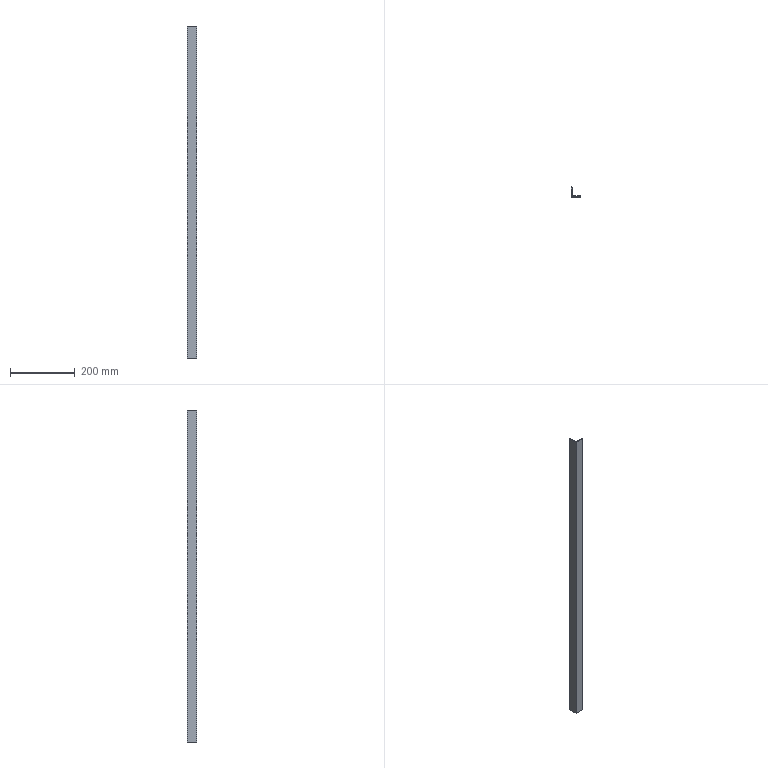Part | SolidWorks | features Extrusion 1 | 1 solid | 11 faces | box 30 x 30 x 1024 mm | volume 174225 mm3 | plane 8 | cylinder 3 | commonest cylinder face diameters 4 x3
STEP:
#1=CARTESIAN_POINT('',(0.,30.,0.));
#2=VERTEX_POINT('',#1);
#3=CARTESIAN_POINT('',(0.,0.,0.));
#4=VERTEX_POINT('',#3);
#5=CARTESIAN_POINT('',(0.,0.,0.));
#6=DIRECTION('',(0.,-1.,0.));
#7=VECTOR('',#6,1000.);
#8=LINE('',#5,#7);
#9=EDGE_CURVE('',#2,#4,#8,.T.);
#10=ORIENTED_EDGE('',*,*,#9,.T.);
#11=CARTESIAN_POINT('',(0.,0.,1024.));
#12=VERTEX_POINT('',#11);
#13=CARTESIAN_POINT('',(0.,0.,1024.));
#14=DIRECTION('',(0.,0.,-1.));
#15=VECTOR('',#14,1000.);
#16=LINE('',#13,#15);
#17=EDGE_CURVE('',#12,#4,#16,.T.);
#18=ORIENTED_EDGE('',*,*,#17,.F.);
#19=CARTESIAN_POINT('',(0.,30.,1024.));
#20=VERTEX_POINT('',#19);
#21=CARTESIAN_POINT('',(0.,0.,1024.));
#22=DIRECTION('',(0.,-1.,0.));
#23=VECTOR('',#22,1000.);
#24=LINE('',#21,#23);
#25=EDGE_CURVE('',#20,#12,#24,.T.);
#26=ORIENTED_EDGE('',*,*,#25,.F.);
#27=CARTESIAN_POINT('',(0.,30.,1024.));
#28=DIRECTION('',(0.,0.,-1.));
#29=VECTOR('',#28,1000.);
#30=LINE('',#27,#29);
#31=EDGE_CURVE('',#20,#2,#30,.T.);
#32=ORIENTED_EDGE('',*,*,#31,.T.);
#33=EDGE_LOOP('',(#10,#18,#26,#32));
#34=FACE_OUTER_BOUND('',#33,.T.);
#35=CARTESIAN_POINT('',(0.,0.,1024.));
#36=DIRECTION('',(1.,0.,0.));
#37=DIRECTION('',(0.,0.,-1.));
#38=AXIS2_PLACEMENT_3D('',#35,#36,#37);
#39=PLANE('',#38);
#40=ADVANCED_FACE('',(#34),#39,.F.);
#41=CARTESIAN_POINT('',(30.,0.,0.));
#42=VERTEX_POINT('',#41);
#43=CARTESIAN_POINT('',(0.,0.,0.));
#44=DIRECTION('',(1.,0.,0.));
#45=VECTOR('',#44,1000.);
#46=LINE('',#43,#45);
#47=EDGE_CURVE('',#4,#42,#46,.T.);
#48=ORIENTED_EDGE('',*,*,#47,.T.);
#49=CARTESIAN_POINT('',(30.,0.,1024.));
#50=VERTEX_POINT('',#49);
#51=CARTESIAN_POINT('',(30.,0.,1024.));
#52=DIRECTION('',(0.,0.,-1.));
#53=VECTOR('',#52,1000.);
#54=LINE('',#51,#53);
#55=EDGE_CURVE('',#50,#42,#54,.T.);
#56=ORIENTED_EDGE('',*,*,#55,.F.);
#57=CARTESIAN_POINT('',(0.,0.,1024.));
#58=DIRECTION('',(1.,0.,0.));
#59=VECTOR('',#58,1000.);
#60=LINE('',#57,#59);
#61=EDGE_CURVE('',#12,#50,#60,.T.);
#62=ORIENTED_EDGE('',*,*,#61,.F.);
#63=ORIENTED_EDGE('',*,*,#17,.T.);
#64=EDGE_LOOP('',(#48,#56,#62,#63));
#65=FACE_OUTER_BOUND('',#64,.T.);
#66=CARTESIAN_POINT('',(0.,0.,1024.));
#67=DIRECTION('',(0.,1.,0.));
#68=DIRECTION('',(0.,0.,1.));
#69=AXIS2_PLACEMENT_3D('',#66,#67,#68);
#70=PLANE('',#69);
#71=ADVANCED_FACE('',(#65),#70,.F.);
#72=CARTESIAN_POINT('',(30.,1.,0.));
#73=VERTEX_POINT('',#72);
#74=CARTESIAN_POINT('',(30.,1.,0.));
#75=DIRECTION('',(0.,1.,0.));
#76=VECTOR('',#75,1000.);
#77=LINE('',#74,#76);
#78=EDGE_CURVE('',#42,#73,#77,.T.);
#79=ORIENTED_EDGE('',*,*,#78,.T.);
#80=CARTESIAN_POINT('',(30.,1.,1024.));
#81=VERTEX_POINT('',#80);
#82=CARTESIAN_POINT('',(30.,1.,1024.));
#83=DIRECTION('',(0.,0.,-1.));
#84=VECTOR('',#83,1000.);
#85=LINE('',#82,#84);
#86=EDGE_CURVE('',#81,#73,#85,.T.);
#87=ORIENTED_EDGE('',*,*,#86,.F.);
#88=CARTESIAN_POINT('',(30.,1.,1024.));
#89=DIRECTION('',(0.,1.,0.));
#90=VECTOR('',#89,1000.);
#91=LINE('',#88,#90);
#92=EDGE_CURVE('',#50,#81,#91,.T.);
#93=ORIENTED_EDGE('',*,*,#92,.F.);
#94=ORIENTED_EDGE('',*,*,#55,.T.);
#95=EDGE_LOOP('',(#79,#87,#93,#94));
#96=FACE_OUTER_BOUND('',#95,.T.);
#97=CARTESIAN_POINT('',(30.,1.,1024.));
#98=DIRECTION('',(-1.,0.,0.));
#99=DIRECTION('',(0.,0.,1.));
#100=AXIS2_PLACEMENT_3D('',#97,#98,#99);
#101=PLANE('',#100);
#102=ADVANCED_FACE('',(#96),#101,.F.);
#103=CARTESIAN_POINT('',(28.,3.,0.));
#104=VERTEX_POINT('',#103);
#105=CARTESIAN_POINT('',(28.,1.,0.));
#106=DIRECTION('',(0.,0.,1.));
#107=DIRECTION('',(1.,0.,0.));
#108=AXIS2_PLACEMENT_3D('',#105,#106,#107);
#109=CIRCLE('',#108,2.);
#110=EDGE_CURVE('',#73,#104,#109,.T.);
#111=ORIENTED_EDGE('',*,*,#110,.T.);
#112=CARTESIAN_POINT('',(28.,3.,1024.));
#113=VERTEX_POINT('',#112);
#114=CARTESIAN_POINT('',(28.,3.,1024.));
#115=DIRECTION('',(0.,0.,-1.));
#116=VECTOR('',#115,1000.);
#117=LINE('',#114,#116);
#118=EDGE_CURVE('',#113,#104,#117,.T.);
#119=ORIENTED_EDGE('',*,*,#118,.F.);
#120=CARTESIAN_POINT('',(28.,1.,1024.));
#121=DIRECTION('',(0.,0.,1.));
#122=DIRECTION('',(1.,0.,0.));
#123=AXIS2_PLACEMENT_3D('',#120,#121,#122);
#124=CIRCLE('',#123,2.);
#125=EDGE_CURVE('',#81,#113,#124,.T.);
#126=ORIENTED_EDGE('',*,*,#125,.F.);
#127=ORIENTED_EDGE('',*,*,#86,.T.);
#128=EDGE_LOOP('',(#111,#119,#126,#127));
#129=FACE_OUTER_BOUND('',#128,.T.);
#130=CARTESIAN_POINT('',(28.,1.,1024.));
#131=DIRECTION('',(0.,0.,-1.));
#132=DIRECTION('',(-1.,0.,0.));
#133=AXIS2_PLACEMENT_3D('',#130,#131,#132);
#134=CYLINDRICAL_SURFACE('',#133,2.);
#135=ADVANCED_FACE('',(#129),#134,.T.);
#136=CARTESIAN_POINT('',(5.,3.,0.));
#137=VERTEX_POINT('',#136);
#138=CARTESIAN_POINT('',(5.,3.,0.));
#139=DIRECTION('',(-1.,0.,0.));
#140=VECTOR('',#139,1000.);
#141=LINE('',#138,#140);
#142=EDGE_CURVE('',#104,#137,#141,.T.);
#143=ORIENTED_EDGE('',*,*,#142,.T.);
#144=CARTESIAN_POINT('',(5.,3.,1024.));
#145=VERTEX_POINT('',#144);
#146=CARTESIAN_POINT('',(5.,3.,1024.));
#147=DIRECTION('',(0.,0.,-1.));
#148=VECTOR('',#147,1000.);
#149=LINE('',#146,#148);
#150=EDGE_CURVE('',#145,#137,#149,.T.);
#151=ORIENTED_EDGE('',*,*,#150,.F.);
#152=CARTESIAN_POINT('',(5.,3.,1024.));
#153=DIRECTION('',(-1.,0.,0.));
#154=VECTOR('',#153,1000.);
#155=LINE('',#152,#154);
#156=EDGE_CURVE('',#113,#145,#155,.T.);
#157=ORIENTED_EDGE('',*,*,#156,.F.);
#158=ORIENTED_EDGE('',*,*,#118,.T.);
#159=EDGE_LOOP('',(#143,#151,#157,#158));
#160=FACE_OUTER_BOUND('',#159,.T.);
#161=CARTESIAN_POINT('',(5.,3.,1024.));
#162=DIRECTION('',(0.,-1.,0.));
#163=DIRECTION('',(0.,0.,-1.));
#164=AXIS2_PLACEMENT_3D('',#161,#162,#163);
#165=PLANE('',#164);
#166=ADVANCED_FACE('',(#160),#165,.F.);
#167=CARTESIAN_POINT('',(3.,5.,0.));
#168=VERTEX_POINT('',#167);
#169=CARTESIAN_POINT('',(5.,5.,0.));
#170=DIRECTION('',(0.,0.,-1.));
#171=DIRECTION('',(-1.,0.,0.));
#172=AXIS2_PLACEMENT_3D('',#169,#170,#171);
#173=CIRCLE('',#172,2.);
#174=EDGE_CURVE('',#137,#168,#173,.T.);
#175=ORIENTED_EDGE('',*,*,#174,.T.);
#176=CARTESIAN_POINT('',(3.,5.,1024.));
#177=VERTEX_POINT('',#176);
#178=CARTESIAN_POINT('',(3.,5.,1024.));
#179=DIRECTION('',(0.,0.,-1.));
#180=VECTOR('',#179,1000.);
#181=LINE('',#178,#180);
#182=EDGE_CURVE('',#177,#168,#181,.T.);
#183=ORIENTED_EDGE('',*,*,#182,.F.);
#184=CARTESIAN_POINT('',(5.,5.,1024.));
#185=DIRECTION('',(0.,0.,-1.));
#186=DIRECTION('',(-1.,0.,0.));
#187=AXIS2_PLACEMENT_3D('',#184,#185,#186);
#188=CIRCLE('',#187,2.);
#189=EDGE_CURVE('',#145,#177,#188,.T.);
#190=ORIENTED_EDGE('',*,*,#189,.F.);
#191=ORIENTED_EDGE('',*,*,#150,.T.);
#192=EDGE_LOOP('',(#175,#183,#190,#191));
#193=FACE_OUTER_BOUND('',#192,.T.);
#194=CARTESIAN_POINT('',(5.,5.,1024.));
#195=DIRECTION('',(0.,0.,-1.));
#196=DIRECTION('',(-1.,0.,0.));
#197=AXIS2_PLACEMENT_3D('',#194,#195,#196);
#198=CYLINDRICAL_SURFACE('',#197,2.);
#199=ADVANCED_FACE('',(#193),#198,.F.);
#200=CARTESIAN_POINT('',(3.,28.,0.));
#201=VERTEX_POINT('',#200);
#202=CARTESIAN_POINT('',(3.,5.,0.));
#203=DIRECTION('',(0.,1.,0.));
#204=VECTOR('',#203,1000.);
#205=LINE('',#202,#204);
#206=EDGE_CURVE('',#168,#201,#205,.T.);
#207=ORIENTED_EDGE('',*,*,#206,.T.);
#208=CARTESIAN_POINT('',(3.,28.,1024.));
#209=VERTEX_POINT('',#208);
#210=CARTESIAN_POINT('',(3.,28.,1024.));
#211=DIRECTION('',(0.,0.,-1.));
#212=VECTOR('',#211,1000.);
#213=LINE('',#210,#212);
#214=EDGE_CURVE('',#209,#201,#213,.T.);
#215=ORIENTED_EDGE('',*,*,#214,.F.);
#216=CARTESIAN_POINT('',(3.,5.,1024.));
#217=DIRECTION('',(0.,1.,0.));
#218=VECTOR('',#217,1000.);
#219=LINE('',#216,#218);
#220=EDGE_CURVE('',#177,#209,#219,.T.);
#221=ORIENTED_EDGE('',*,*,#220,.F.);
#222=ORIENTED_EDGE('',*,*,#182,.T.);
#223=EDGE_LOOP('',(#207,#215,#221,#222));
#224=FACE_OUTER_BOUND('',#223,.T.);
#225=CARTESIAN_POINT('',(3.,5.,1024.));
#226=DIRECTION('',(-1.,0.,0.));
#227=DIRECTION('',(0.,0.,1.));
#228=AXIS2_PLACEMENT_3D('',#225,#226,#227);
#229=PLANE('',#228);
#230=ADVANCED_FACE('',(#224),#229,.F.);
#231=CARTESIAN_POINT('',(1.,30.,0.));
#232=VERTEX_POINT('',#231);
#233=CARTESIAN_POINT('',(1.,28.,0.));
#234=DIRECTION('',(0.,0.,1.));
#235=DIRECTION('',(1.,0.,0.));
#236=AXIS2_PLACEMENT_3D('',#233,#234,#235);
#237=CIRCLE('',#236,2.);
#238=EDGE_CURVE('',#201,#232,#237,.T.);
#239=ORIENTED_EDGE('',*,*,#238,.T.);
#240=CARTESIAN_POINT('',(1.,30.,1024.));
#241=VERTEX_POINT('',#240);
#242=CARTESIAN_POINT('',(1.,30.,1024.));
#243=DIRECTION('',(0.,0.,-1.));
#244=VECTOR('',#243,1000.);
#245=LINE('',#242,#244);
#246=EDGE_CURVE('',#241,#232,#245,.T.);
#247=ORIENTED_EDGE('',*,*,#246,.F.);
#248=CARTESIAN_POINT('',(1.,28.,1024.));
#249=DIRECTION('',(0.,0.,1.));
#250=DIRECTION('',(1.,0.,0.));
#251=AXIS2_PLACEMENT_3D('',#248,#249,#250);
#252=CIRCLE('',#251,2.);
#253=EDGE_CURVE('',#209,#241,#252,.T.);
#254=ORIENTED_EDGE('',*,*,#253,.F.);
#255=ORIENTED_EDGE('',*,*,#214,.T.);
#256=EDGE_LOOP('',(#239,#247,#254,#255));
#257=FACE_OUTER_BOUND('',#256,.T.);
#258=CARTESIAN_POINT('',(1.,28.,1024.));
#259=DIRECTION('',(0.,0.,-1.));
#260=DIRECTION('',(-1.,0.,0.));
#261=AXIS2_PLACEMENT_3D('',#258,#259,#260);
#262=CYLINDRICAL_SURFACE('',#261,2.);
#263=ADVANCED_FACE('',(#257),#262,.T.);
#264=CARTESIAN_POINT('',(0.,30.,0.));
#265=DIRECTION('',(-1.,0.,0.));
#266=VECTOR('',#265,1000.);
#267=LINE('',#264,#266);
#268=EDGE_CURVE('',#232,#2,#267,.T.);
#269=ORIENTED_EDGE('',*,*,#268,.T.);
#270=ORIENTED_EDGE('',*,*,#31,.F.);
#271=CARTESIAN_POINT('',(0.,30.,1024.));
#272=DIRECTION('',(-1.,0.,0.));
#273=VECTOR('',#272,1000.);
#274=LINE('',#271,#273);
#275=EDGE_CURVE('',#241,#20,#274,.T.);
#276=ORIENTED_EDGE('',*,*,#275,.F.);
#277=ORIENTED_EDGE('',*,*,#246,.T.);
#278=EDGE_LOOP('',(#269,#270,#276,#277));
#279=FACE_OUTER_BOUND('',#278,.T.);
#280=CARTESIAN_POINT('',(0.,30.,1024.));
#281=DIRECTION('',(0.,-1.,0.));
#282=DIRECTION('',(0.,0.,-1.));
#283=AXIS2_PLACEMENT_3D('',#280,#281,#282);
#284=PLANE('',#283);
#285=ADVANCED_FACE('',(#279),#284,.F.);
#286=ORIENTED_EDGE('',*,*,#25,.T.);
#287=ORIENTED_EDGE('',*,*,#61,.T.);
#288=ORIENTED_EDGE('',*,*,#92,.T.);
#289=ORIENTED_EDGE('',*,*,#125,.T.);
#290=ORIENTED_EDGE('',*,*,#156,.T.);
#291=ORIENTED_EDGE('',*,*,#189,.T.);
#292=ORIENTED_EDGE('',*,*,#220,.T.);
#293=ORIENTED_EDGE('',*,*,#253,.T.);
#294=ORIENTED_EDGE('',*,*,#275,.T.);
#295=EDGE_LOOP('',(#286,#287,#288,#289,#290,#291,#292,#293,#294));
#296=FACE_OUTER_BOUND('',#295,.T.);
#297=CARTESIAN_POINT('',(1.,28.,1024.));
#298=DIRECTION('',(0.,0.,1.));
#299=DIRECTION('',(1.,0.,0.));
#300=AXIS2_PLACEMENT_3D('',#297,#298,#299);
#301=PLANE('',#300);
#302=ADVANCED_FACE('',(#296),#301,.T.);
#303=ORIENTED_EDGE('',*,*,#9,.F.);
#304=ORIENTED_EDGE('',*,*,#268,.F.);
#305=ORIENTED_EDGE('',*,*,#238,.F.);
#306=ORIENTED_EDGE('',*,*,#206,.F.);
#307=ORIENTED_EDGE('',*,*,#174,.F.);
#308=ORIENTED_EDGE('',*,*,#142,.F.);
#309=ORIENTED_EDGE('',*,*,#110,.F.);
#310=ORIENTED_EDGE('',*,*,#78,.F.);
#311=ORIENTED_EDGE('',*,*,#47,.F.);
#312=EDGE_LOOP('',(#303,#304,#305,#306,#307,#308,#309,#310,#311));
#313=FACE_OUTER_BOUND('',#312,.T.);
#314=CARTESIAN_POINT('',(1.,28.,0.));
#315=DIRECTION('',(0.,0.,1.));
#316=DIRECTION('',(1.,0.,0.));
#317=AXIS2_PLACEMENT_3D('',#314,#315,#316);
#318=PLANE('',#317);
#319=ADVANCED_FACE('',(#313),#318,.F.);
#320=CLOSED_SHELL('',(#40,#71,#102,#135,#166,#199,#230,#263,#285,#302,#319));
#321=MANIFOLD_SOLID_BREP('',#320);
#322=CARTESIAN_POINT('',(0.,0.,0.));
#323=DIRECTION('',(0.,0.,1.));
#324=DIRECTION('',(1.,0.,0.));
#325=AXIS2_PLACEMENT_3D('',#322,#323,#324);
#326=(LENGTH_UNIT()NAMED_UNIT(*)SI_UNIT(.MILLI.,.METRE.));
#327=UNCERTAINTY_MEASURE_WITH_UNIT(LENGTH_MEASURE(0.00001),#326,'','');
#328=(NAMED_UNIT(*)PLANE_ANGLE_UNIT()SI_UNIT($,.RADIAN.));
#329=(NAMED_UNIT(*)SI_UNIT($,.STERADIAN.)SOLID_ANGLE_UNIT());
#330=(GEOMETRIC_REPRESENTATION_CONTEXT(3)GLOBAL_UNCERTAINTY_ASSIGNED_CONTEXT((#327))GLOBAL_UNIT_ASSIGNED_CONTEXT((#326,#328,#329))REPRESENTATION_CONTEXT('',''));
#331=ADVANCED_BREP_SHAPE_REPRESENTATION('',(#321,#325),#330);